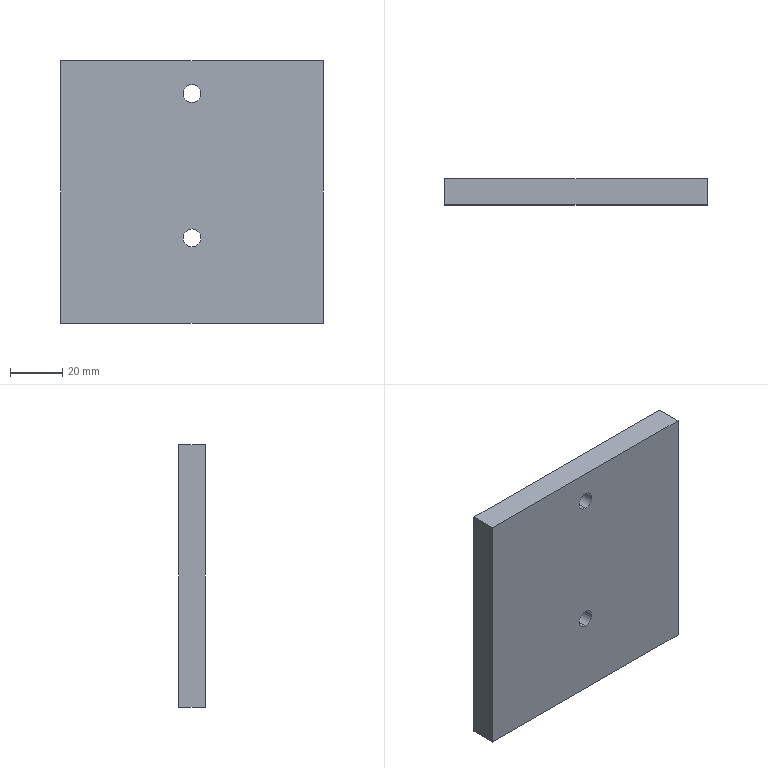Part | SolidWorks | features BaseBody 1 | 1 solid | 10 faces | box 100 x 10 x 100 mm | volume 99274 mm3 | plane 6 | cylinder 4 | commonest cylinder face diameters 6.8 x4
STEP:
#1=CARTESIAN_POINT('',(-400.,2372.,-1335.9));
#2=VERTEX_POINT('',#1);
#3=CARTESIAN_POINT('',(-400.,2372.,-1329.1));
#4=VERTEX_POINT('',#3);
#5=CARTESIAN_POINT('',(-400.,2372.,-1332.5));
#6=DIRECTION('',(0.,1.,0.));
#7=DIRECTION('',(0.,0.,-1.));
#8=AXIS2_PLACEMENT_3D('',#5,#6,#7);
#9=CIRCLE('',#8,3.4);
#10=EDGE_CURVE('',#2,#4,#9,.T.);
#11=ORIENTED_EDGE('',*,*,#10,.T.);
#12=CARTESIAN_POINT('',(-400.,2362.,-1329.1));
#13=VERTEX_POINT('',#12);
#14=CARTESIAN_POINT('',(-400.,2362.,-1329.1));
#15=DIRECTION('',(0.,-1.,0.));
#16=VECTOR('',#15,1000.);
#17=LINE('',#14,#16);
#18=EDGE_CURVE('',#4,#13,#17,.T.);
#19=ORIENTED_EDGE('',*,*,#18,.T.);
#20=CARTESIAN_POINT('',(-400.,2362.,-1335.9));
#21=VERTEX_POINT('',#20);
#22=CARTESIAN_POINT('',(-400.,2362.,-1332.5));
#23=DIRECTION('',(0.,1.,0.));
#24=DIRECTION('',(0.,0.,-1.));
#25=AXIS2_PLACEMENT_3D('',#22,#23,#24);
#26=CIRCLE('',#25,3.4);
#27=EDGE_CURVE('',#21,#13,#26,.T.);
#28=ORIENTED_EDGE('',*,*,#27,.F.);
#29=CARTESIAN_POINT('',(-400.,2362.,-1335.9));
#30=DIRECTION('',(0.,-1.,0.));
#31=VECTOR('',#30,1000.);
#32=LINE('',#29,#31);
#33=EDGE_CURVE('',#2,#21,#32,.T.);
#34=ORIENTED_EDGE('',*,*,#33,.F.);
#35=EDGE_LOOP('',(#11,#19,#28,#34));
#36=FACE_OUTER_BOUND('',#35,.T.);
#37=CARTESIAN_POINT('',(-400.,2362.,-1332.5));
#38=DIRECTION('',(0.,-1.,0.));
#39=DIRECTION('',(0.,0.,-1.));
#40=AXIS2_PLACEMENT_3D('',#37,#38,#39);
#41=CYLINDRICAL_SURFACE('',#40,3.4);
#42=ADVANCED_FACE('',(#36),#41,.F.);
#43=CARTESIAN_POINT('',(-400.,2372.,-1280.9));
#44=VERTEX_POINT('',#43);
#45=CARTESIAN_POINT('',(-400.,2372.,-1274.1));
#46=VERTEX_POINT('',#45);
#47=CARTESIAN_POINT('',(-400.,2372.,-1277.5));
#48=DIRECTION('',(0.,1.,0.));
#49=DIRECTION('',(0.,0.,-1.));
#50=AXIS2_PLACEMENT_3D('',#47,#48,#49);
#51=CIRCLE('',#50,3.4);
#52=EDGE_CURVE('',#44,#46,#51,.T.);
#53=ORIENTED_EDGE('',*,*,#52,.T.);
#54=CARTESIAN_POINT('',(-400.,2362.,-1274.1));
#55=VERTEX_POINT('',#54);
#56=CARTESIAN_POINT('',(-400.,2362.,-1274.1));
#57=DIRECTION('',(0.,-1.,0.));
#58=VECTOR('',#57,1000.);
#59=LINE('',#56,#58);
#60=EDGE_CURVE('',#46,#55,#59,.T.);
#61=ORIENTED_EDGE('',*,*,#60,.T.);
#62=CARTESIAN_POINT('',(-400.,2362.,-1280.9));
#63=VERTEX_POINT('',#62);
#64=CARTESIAN_POINT('',(-400.,2362.,-1277.5));
#65=DIRECTION('',(0.,1.,0.));
#66=DIRECTION('',(0.,0.,-1.));
#67=AXIS2_PLACEMENT_3D('',#64,#65,#66);
#68=CIRCLE('',#67,3.4);
#69=EDGE_CURVE('',#63,#55,#68,.T.);
#70=ORIENTED_EDGE('',*,*,#69,.F.);
#71=CARTESIAN_POINT('',(-400.,2362.,-1280.9));
#72=DIRECTION('',(0.,-1.,0.));
#73=VECTOR('',#72,1000.);
#74=LINE('',#71,#73);
#75=EDGE_CURVE('',#44,#63,#74,.T.);
#76=ORIENTED_EDGE('',*,*,#75,.F.);
#77=EDGE_LOOP('',(#53,#61,#70,#76));
#78=FACE_OUTER_BOUND('',#77,.T.);
#79=CARTESIAN_POINT('',(-400.,2362.,-1277.5));
#80=DIRECTION('',(0.,-1.,0.));
#81=DIRECTION('',(0.,0.,-1.));
#82=AXIS2_PLACEMENT_3D('',#79,#80,#81);
#83=CYLINDRICAL_SURFACE('',#82,3.4);
#84=ADVANCED_FACE('',(#78),#83,.F.);
#85=ORIENTED_EDGE('',*,*,#10,.F.);
#86=CARTESIAN_POINT('',(-400.,2372.,-1332.5));
#87=DIRECTION('',(0.,1.,0.));
#88=DIRECTION('',(0.,0.,-1.));
#89=AXIS2_PLACEMENT_3D('',#86,#87,#88);
#90=CIRCLE('',#89,3.4);
#91=EDGE_CURVE('',#4,#2,#90,.T.);
#92=ORIENTED_EDGE('',*,*,#91,.F.);
#93=EDGE_LOOP('',(#85,#92));
#94=FACE_BOUND('',#93,.T.);
#95=ORIENTED_EDGE('',*,*,#52,.F.);
#96=CARTESIAN_POINT('',(-400.,2372.,-1277.5));
#97=DIRECTION('',(0.,1.,0.));
#98=DIRECTION('',(0.,0.,-1.));
#99=AXIS2_PLACEMENT_3D('',#96,#97,#98);
#100=CIRCLE('',#99,3.4);
#101=EDGE_CURVE('',#46,#44,#100,.T.);
#102=ORIENTED_EDGE('',*,*,#101,.F.);
#103=EDGE_LOOP('',(#95,#102));
#104=FACE_BOUND('',#103,.T.);
#105=CARTESIAN_POINT('',(-350.,2372.,-1265.));
#106=VERTEX_POINT('',#105);
#107=CARTESIAN_POINT('',(-450.,2372.,-1265.));
#108=VERTEX_POINT('',#107);
#109=CARTESIAN_POINT('',(-350.,2372.,-1265.));
#110=DIRECTION('',(-1.,0.,0.));
#111=VECTOR('',#110,1000.);
#112=LINE('',#109,#111);
#113=EDGE_CURVE('',#106,#108,#112,.T.);
#114=ORIENTED_EDGE('',*,*,#113,.F.);
#115=CARTESIAN_POINT('',(-350.,2372.,-1365.));
#116=VERTEX_POINT('',#115);
#117=CARTESIAN_POINT('',(-350.,2372.,-1365.));
#118=DIRECTION('',(0.,0.,1.));
#119=VECTOR('',#118,1000.);
#120=LINE('',#117,#119);
#121=EDGE_CURVE('',#116,#106,#120,.T.);
#122=ORIENTED_EDGE('',*,*,#121,.F.);
#123=CARTESIAN_POINT('',(-450.,2372.,-1365.));
#124=VERTEX_POINT('',#123);
#125=CARTESIAN_POINT('',(-350.,2372.,-1365.));
#126=DIRECTION('',(1.,0.,0.));
#127=VECTOR('',#126,1000.);
#128=LINE('',#125,#127);
#129=EDGE_CURVE('',#124,#116,#128,.T.);
#130=ORIENTED_EDGE('',*,*,#129,.F.);
#131=CARTESIAN_POINT('',(-450.,2372.,-1365.));
#132=DIRECTION('',(0.,0.,-1.));
#133=VECTOR('',#132,1000.);
#134=LINE('',#131,#133);
#135=EDGE_CURVE('',#108,#124,#134,.T.);
#136=ORIENTED_EDGE('',*,*,#135,.F.);
#137=EDGE_LOOP('',(#114,#122,#130,#136));
#138=FACE_OUTER_BOUND('',#137,.T.);
#139=CARTESIAN_POINT('',(-350.,2372.,-1365.));
#140=DIRECTION('',(0.,-1.,0.));
#141=DIRECTION('',(0.,0.,-1.));
#142=AXIS2_PLACEMENT_3D('',#139,#140,#141);
#143=PLANE('',#142);
#144=ADVANCED_FACE('',(#94,#104,#138),#143,.F.);
#145=ORIENTED_EDGE('',*,*,#18,.F.);
#146=ORIENTED_EDGE('',*,*,#91,.T.);
#147=ORIENTED_EDGE('',*,*,#33,.T.);
#148=CARTESIAN_POINT('',(-400.,2362.,-1332.5));
#149=DIRECTION('',(0.,1.,0.));
#150=DIRECTION('',(0.,0.,-1.));
#151=AXIS2_PLACEMENT_3D('',#148,#149,#150);
#152=CIRCLE('',#151,3.4);
#153=EDGE_CURVE('',#13,#21,#152,.T.);
#154=ORIENTED_EDGE('',*,*,#153,.F.);
#155=EDGE_LOOP('',(#145,#146,#147,#154));
#156=FACE_OUTER_BOUND('',#155,.T.);
#157=CARTESIAN_POINT('',(-400.,2362.,-1332.5));
#158=DIRECTION('',(0.,-1.,0.));
#159=DIRECTION('',(0.,0.,-1.));
#160=AXIS2_PLACEMENT_3D('',#157,#158,#159);
#161=CYLINDRICAL_SURFACE('',#160,3.4);
#162=ADVANCED_FACE('',(#156),#161,.F.);
#163=ORIENTED_EDGE('',*,*,#60,.F.);
#164=ORIENTED_EDGE('',*,*,#101,.T.);
#165=ORIENTED_EDGE('',*,*,#75,.T.);
#166=CARTESIAN_POINT('',(-400.,2362.,-1277.5));
#167=DIRECTION('',(0.,1.,0.));
#168=DIRECTION('',(0.,0.,-1.));
#169=AXIS2_PLACEMENT_3D('',#166,#167,#168);
#170=CIRCLE('',#169,3.4);
#171=EDGE_CURVE('',#55,#63,#170,.T.);
#172=ORIENTED_EDGE('',*,*,#171,.F.);
#173=EDGE_LOOP('',(#163,#164,#165,#172));
#174=FACE_OUTER_BOUND('',#173,.T.);
#175=CARTESIAN_POINT('',(-400.,2362.,-1277.5));
#176=DIRECTION('',(0.,-1.,0.));
#177=DIRECTION('',(0.,0.,-1.));
#178=AXIS2_PLACEMENT_3D('',#175,#176,#177);
#179=CYLINDRICAL_SURFACE('',#178,3.4);
#180=ADVANCED_FACE('',(#174),#179,.F.);
#181=CARTESIAN_POINT('',(-450.,2362.,-1265.));
#182=VERTEX_POINT('',#181);
#183=CARTESIAN_POINT('',(-450.,2362.,-1365.));
#184=VERTEX_POINT('',#183);
#185=CARTESIAN_POINT('',(-450.,2362.,-1365.));
#186=DIRECTION('',(0.,0.,-1.));
#187=VECTOR('',#186,1000.);
#188=LINE('',#185,#187);
#189=EDGE_CURVE('',#182,#184,#188,.T.);
#190=ORIENTED_EDGE('',*,*,#189,.F.);
#191=CARTESIAN_POINT('',(-450.,2362.,-1265.));
#192=DIRECTION('',(0.,-1.,0.));
#193=VECTOR('',#192,1000.);
#194=LINE('',#191,#193);
#195=EDGE_CURVE('',#108,#182,#194,.T.);
#196=ORIENTED_EDGE('',*,*,#195,.F.);
#197=ORIENTED_EDGE('',*,*,#135,.T.);
#198=CARTESIAN_POINT('',(-450.,2362.,-1365.));
#199=DIRECTION('',(0.,1.,0.));
#200=VECTOR('',#199,1000.);
#201=LINE('',#198,#200);
#202=EDGE_CURVE('',#184,#124,#201,.T.);
#203=ORIENTED_EDGE('',*,*,#202,.F.);
#204=EDGE_LOOP('',(#190,#196,#197,#203));
#205=FACE_OUTER_BOUND('',#204,.T.);
#206=CARTESIAN_POINT('',(-450.,2362.,-1365.));
#207=DIRECTION('',(1.,0.,0.));
#208=DIRECTION('',(0.,0.,-1.));
#209=AXIS2_PLACEMENT_3D('',#206,#207,#208);
#210=PLANE('',#209);
#211=ADVANCED_FACE('',(#205),#210,.F.);
#212=CARTESIAN_POINT('',(-350.,2362.,-1265.));
#213=VERTEX_POINT('',#212);
#214=CARTESIAN_POINT('',(-450.,2362.,-1265.));
#215=DIRECTION('',(-1.,0.,0.));
#216=VECTOR('',#215,1000.);
#217=LINE('',#214,#216);
#218=EDGE_CURVE('',#213,#182,#217,.T.);
#219=ORIENTED_EDGE('',*,*,#218,.F.);
#220=CARTESIAN_POINT('',(-350.,2362.,-1265.));
#221=DIRECTION('',(0.,-1.,0.));
#222=VECTOR('',#221,1000.);
#223=LINE('',#220,#222);
#224=EDGE_CURVE('',#106,#213,#223,.T.);
#225=ORIENTED_EDGE('',*,*,#224,.F.);
#226=ORIENTED_EDGE('',*,*,#113,.T.);
#227=ORIENTED_EDGE('',*,*,#195,.T.);
#228=EDGE_LOOP('',(#219,#225,#226,#227));
#229=FACE_OUTER_BOUND('',#228,.T.);
#230=CARTESIAN_POINT('',(-450.,2362.,-1265.));
#231=DIRECTION('',(0.,0.,-1.));
#232=DIRECTION('',(-1.,0.,0.));
#233=AXIS2_PLACEMENT_3D('',#230,#231,#232);
#234=PLANE('',#233);
#235=ADVANCED_FACE('',(#229),#234,.F.);
#236=CARTESIAN_POINT('',(-350.,2362.,-1365.));
#237=VERTEX_POINT('',#236);
#238=CARTESIAN_POINT('',(-350.,2362.,-1365.));
#239=DIRECTION('',(0.,0.,1.));
#240=VECTOR('',#239,1000.);
#241=LINE('',#238,#240);
#242=EDGE_CURVE('',#237,#213,#241,.T.);
#243=ORIENTED_EDGE('',*,*,#242,.F.);
#244=CARTESIAN_POINT('',(-350.,2362.,-1365.));
#245=DIRECTION('',(0.,-1.,0.));
#246=VECTOR('',#245,1000.);
#247=LINE('',#244,#246);
#248=EDGE_CURVE('',#116,#237,#247,.T.);
#249=ORIENTED_EDGE('',*,*,#248,.F.);
#250=ORIENTED_EDGE('',*,*,#121,.T.);
#251=ORIENTED_EDGE('',*,*,#224,.T.);
#252=EDGE_LOOP('',(#243,#249,#250,#251));
#253=FACE_OUTER_BOUND('',#252,.T.);
#254=CARTESIAN_POINT('',(-350.,2362.,-1365.));
#255=DIRECTION('',(-1.,0.,0.));
#256=DIRECTION('',(0.,0.,1.));
#257=AXIS2_PLACEMENT_3D('',#254,#255,#256);
#258=PLANE('',#257);
#259=ADVANCED_FACE('',(#253),#258,.F.);
#260=CARTESIAN_POINT('',(-450.,2362.,-1365.));
#261=DIRECTION('',(1.,0.,0.));
#262=VECTOR('',#261,1000.);
#263=LINE('',#260,#262);
#264=EDGE_CURVE('',#184,#237,#263,.T.);
#265=ORIENTED_EDGE('',*,*,#264,.F.);
#266=ORIENTED_EDGE('',*,*,#202,.T.);
#267=ORIENTED_EDGE('',*,*,#129,.T.);
#268=ORIENTED_EDGE('',*,*,#248,.T.);
#269=EDGE_LOOP('',(#265,#266,#267,#268));
#270=FACE_OUTER_BOUND('',#269,.T.);
#271=CARTESIAN_POINT('',(-450.,2362.,-1365.));
#272=DIRECTION('',(0.,0.,1.));
#273=DIRECTION('',(1.,0.,0.));
#274=AXIS2_PLACEMENT_3D('',#271,#272,#273);
#275=PLANE('',#274);
#276=ADVANCED_FACE('',(#270),#275,.F.);
#277=ORIENTED_EDGE('',*,*,#27,.T.);
#278=ORIENTED_EDGE('',*,*,#153,.T.);
#279=EDGE_LOOP('',(#277,#278));
#280=FACE_BOUND('',#279,.T.);
#281=ORIENTED_EDGE('',*,*,#69,.T.);
#282=ORIENTED_EDGE('',*,*,#171,.T.);
#283=EDGE_LOOP('',(#281,#282));
#284=FACE_BOUND('',#283,.T.);
#285=ORIENTED_EDGE('',*,*,#189,.T.);
#286=ORIENTED_EDGE('',*,*,#264,.T.);
#287=ORIENTED_EDGE('',*,*,#242,.T.);
#288=ORIENTED_EDGE('',*,*,#218,.T.);
#289=EDGE_LOOP('',(#285,#286,#287,#288));
#290=FACE_OUTER_BOUND('',#289,.T.);
#291=CARTESIAN_POINT('',(-350.,2362.,-1365.));
#292=DIRECTION('',(0.,-1.,0.));
#293=DIRECTION('',(0.,0.,-1.));
#294=AXIS2_PLACEMENT_3D('',#291,#292,#293);
#295=PLANE('',#294);
#296=ADVANCED_FACE('',(#280,#284,#290),#295,.T.);
#297=CLOSED_SHELL('',(#42,#84,#144,#162,#180,#211,#235,#259,#276,#296));
#298=MANIFOLD_SOLID_BREP('',#297);
#299=CARTESIAN_POINT('',(0.,0.,0.));
#300=DIRECTION('',(0.,0.,1.));
#301=DIRECTION('',(1.,0.,0.));
#302=AXIS2_PLACEMENT_3D('',#299,#300,#301);
#303=(LENGTH_UNIT()NAMED_UNIT(*)SI_UNIT(.MILLI.,.METRE.));
#304=UNCERTAINTY_MEASURE_WITH_UNIT(LENGTH_MEASURE(0.00001),#303,'','');
#305=(NAMED_UNIT(*)PLANE_ANGLE_UNIT()SI_UNIT($,.RADIAN.));
#306=(NAMED_UNIT(*)SI_UNIT($,.STERADIAN.)SOLID_ANGLE_UNIT());
#307=(GEOMETRIC_REPRESENTATION_CONTEXT(3)GLOBAL_UNCERTAINTY_ASSIGNED_CONTEXT((#304))GLOBAL_UNIT_ASSIGNED_CONTEXT((#303,#305,#306))REPRESENTATION_CONTEXT('',''));
#308=ADVANCED_BREP_SHAPE_REPRESENTATION('',(#298,#302),#307);